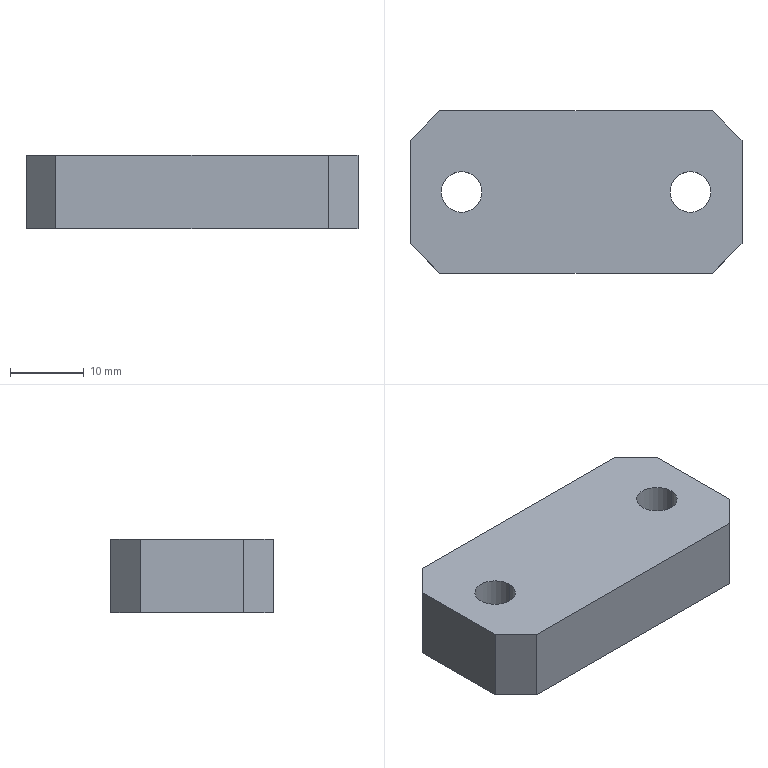Part | Creo | 1 solid | 20 faces | box 45 x 22 x 10 mm | volume 8539 mm3 | plane 12 | cylinder 8 | commonest cylinder face diameters 5.5 x4 9.5 x4
STEP:
#1=CARTESIAN_POINT('',(-202.734,-76.26,-294.5));
#2=VERTEX_POINT('',#1);
#3=CARTESIAN_POINT('',(-165.734,-76.26,-294.5));
#4=VERTEX_POINT('',#3);
#5=CARTESIAN_POINT('',(-202.734,-76.26,-294.5));
#6=DIRECTION('',(1.,0.,0.));
#7=VECTOR('',#6,37.);
#8=LINE('',#5,#7);
#9=EDGE_CURVE('',#2,#4,#8,.T.);
#10=ORIENTED_EDGE('',*,*,#9,.F.);
#11=CARTESIAN_POINT('',(-206.734,-72.26,-294.5));
#12=VERTEX_POINT('',#11);
#13=CARTESIAN_POINT('',(-206.734,-72.26,-294.5));
#14=DIRECTION('',(0.7071,-0.7071,0.));
#15=VECTOR('',#14,5.657);
#16=LINE('',#13,#15);
#17=EDGE_CURVE('',#12,#2,#16,.T.);
#18=ORIENTED_EDGE('',*,*,#17,.F.);
#19=CARTESIAN_POINT('',(-206.734,-58.26,-294.5));
#20=VERTEX_POINT('',#19);
#21=CARTESIAN_POINT('',(-206.734,-72.26,-294.5));
#22=DIRECTION('',(0.,1.,0.));
#23=VECTOR('',#22,14.);
#24=LINE('',#21,#23);
#25=EDGE_CURVE('',#12,#20,#24,.T.);
#26=ORIENTED_EDGE('',*,*,#25,.T.);
#27=CARTESIAN_POINT('',(-202.734,-54.26,-294.5));
#28=VERTEX_POINT('',#27);
#29=CARTESIAN_POINT('',(-202.734,-54.26,-294.5));
#30=DIRECTION('',(-0.7071,-0.7071,0.));
#31=VECTOR('',#30,5.657);
#32=LINE('',#29,#31);
#33=EDGE_CURVE('',#28,#20,#32,.T.);
#34=ORIENTED_EDGE('',*,*,#33,.F.);
#35=CARTESIAN_POINT('',(-165.734,-54.26,-294.5));
#36=VERTEX_POINT('',#35);
#37=CARTESIAN_POINT('',(-165.734,-54.26,-294.5));
#38=DIRECTION('',(-1.,0.,0.));
#39=VECTOR('',#38,37.);
#40=LINE('',#37,#39);
#41=EDGE_CURVE('',#36,#28,#40,.T.);
#42=ORIENTED_EDGE('',*,*,#41,.F.);
#43=CARTESIAN_POINT('',(-161.734,-58.26,-294.5));
#44=VERTEX_POINT('',#43);
#45=CARTESIAN_POINT('',(-161.734,-58.26,-294.5));
#46=DIRECTION('',(-0.7071,0.7071,0.));
#47=VECTOR('',#46,5.657);
#48=LINE('',#45,#47);
#49=EDGE_CURVE('',#44,#36,#48,.T.);
#50=ORIENTED_EDGE('',*,*,#49,.F.);
#51=CARTESIAN_POINT('',(-161.734,-72.26,-294.5));
#52=VERTEX_POINT('',#51);
#53=CARTESIAN_POINT('',(-161.734,-72.26,-294.5));
#54=DIRECTION('',(0.,1.,0.));
#55=VECTOR('',#54,14.);
#56=LINE('',#53,#55);
#57=EDGE_CURVE('',#52,#44,#56,.T.);
#58=ORIENTED_EDGE('',*,*,#57,.F.);
#59=CARTESIAN_POINT('',(-165.734,-76.26,-294.5));
#60=DIRECTION('',(0.7071,0.7071,0.));
#61=VECTOR('',#60,5.657);
#62=LINE('',#59,#61);
#63=EDGE_CURVE('',#4,#52,#62,.T.);
#64=ORIENTED_EDGE('',*,*,#63,.F.);
#65=EDGE_LOOP('',(#10,#18,#26,#34,#42,#50,#58,#64));
#66=FACE_OUTER_BOUND('',#65,.F.);
#67=CARTESIAN_POINT('',(-196.984,-65.26,-294.5));
#68=VERTEX_POINT('',#67);
#69=CARTESIAN_POINT('',(-202.484,-65.26,-294.5));
#70=VERTEX_POINT('',#69);
#71=CARTESIAN_POINT('',(-199.734,-65.26,-294.5));
#72=DIRECTION('',(0.,0.,-1.));
#73=DIRECTION('',(1.,0.,0.));
#74=AXIS2_PLACEMENT_3D('',#71,#72,#73);
#75=CIRCLE('',#74,2.75);
#76=EDGE_CURVE('',#68,#70,#75,.T.);
#77=ORIENTED_EDGE('',*,*,#76,.F.);
#78=CARTESIAN_POINT('',(-199.734,-65.26,-294.5));
#79=DIRECTION('',(0.,0.,-1.));
#80=DIRECTION('',(-1.,0.,0.));
#81=AXIS2_PLACEMENT_3D('',#78,#79,#80);
#82=CIRCLE('',#81,2.75);
#83=EDGE_CURVE('',#70,#68,#82,.T.);
#84=ORIENTED_EDGE('',*,*,#83,.F.);
#85=EDGE_LOOP('',(#77,#84));
#86=FACE_BOUND('',#85,.F.);
#87=CARTESIAN_POINT('',(-165.984,-65.26,-294.5));
#88=VERTEX_POINT('',#87);
#89=CARTESIAN_POINT('',(-171.484,-65.26,-294.5));
#90=VERTEX_POINT('',#89);
#91=CARTESIAN_POINT('',(-168.734,-65.26,-294.5));
#92=DIRECTION('',(0.,0.,-1.));
#93=DIRECTION('',(1.,0.,0.));
#94=AXIS2_PLACEMENT_3D('',#91,#92,#93);
#95=CIRCLE('',#94,2.75);
#96=EDGE_CURVE('',#88,#90,#95,.T.);
#97=ORIENTED_EDGE('',*,*,#96,.F.);
#98=CARTESIAN_POINT('',(-168.734,-65.26,-294.5));
#99=DIRECTION('',(0.,0.,-1.));
#100=DIRECTION('',(-1.,0.,0.));
#101=AXIS2_PLACEMENT_3D('',#98,#99,#100);
#102=CIRCLE('',#101,2.75);
#103=EDGE_CURVE('',#90,#88,#102,.T.);
#104=ORIENTED_EDGE('',*,*,#103,.F.);
#105=EDGE_LOOP('',(#97,#104));
#106=FACE_BOUND('',#105,.F.);
#107=CARTESIAN_POINT('',(-177.734,-55.26,-294.5));
#108=DIRECTION('',(0.,0.,1.));
#109=DIRECTION('',(-1.,0.,0.));
#110=AXIS2_PLACEMENT_3D('',#107,#108,#109);
#111=PLANE('',#110);
#112=ADVANCED_FACE('',(#66,#86,#106),#111,.T.);
#113=CARTESIAN_POINT('',(-202.484,-65.26,-298.5));
#114=VERTEX_POINT('',#113);
#115=CARTESIAN_POINT('',(-196.984,-65.26,-298.5));
#116=VERTEX_POINT('',#115);
#117=CARTESIAN_POINT('',(-199.734,-65.26,-298.5));
#118=DIRECTION('',(0.,0.,1.));
#119=DIRECTION('',(-1.,0.,0.));
#120=AXIS2_PLACEMENT_3D('',#117,#118,#119);
#121=CIRCLE('',#120,2.75);
#122=EDGE_CURVE('',#114,#116,#121,.T.);
#123=ORIENTED_EDGE('',*,*,#122,.T.);
#124=CARTESIAN_POINT('',(-196.984,-65.26,-294.5));
#125=DIRECTION('',(0.,0.,-1.));
#126=VECTOR('',#125,4.);
#127=LINE('',#124,#126);
#128=EDGE_CURVE('',#68,#116,#127,.T.);
#129=ORIENTED_EDGE('',*,*,#128,.F.);
#130=ORIENTED_EDGE('',*,*,#76,.T.);
#131=CARTESIAN_POINT('',(-202.484,-65.26,-294.5));
#132=DIRECTION('',(0.,0.,-1.));
#133=VECTOR('',#132,4.);
#134=LINE('',#131,#133);
#135=EDGE_CURVE('',#70,#114,#134,.T.);
#136=ORIENTED_EDGE('',*,*,#135,.T.);
#137=EDGE_LOOP('',(#123,#129,#130,#136));
#138=FACE_OUTER_BOUND('',#137,.F.);
#139=CARTESIAN_POINT('',(-199.734,-65.26,-294.5));
#140=DIRECTION('',(0.,0.,-1.));
#141=DIRECTION('',(1.,0.,0.));
#142=AXIS2_PLACEMENT_3D('',#139,#140,#141);
#143=CYLINDRICAL_SURFACE('',#142,2.75);
#144=ADVANCED_FACE('',(#138),#143,.F.);
#145=CARTESIAN_POINT('',(-194.984,-65.26,-298.5));
#146=VERTEX_POINT('',#145);
#147=CARTESIAN_POINT('',(-204.484,-65.26,-298.5));
#148=VERTEX_POINT('',#147);
#149=CARTESIAN_POINT('',(-199.734,-65.26,-298.5));
#150=DIRECTION('',(0.,0.,-1.));
#151=DIRECTION('',(1.,0.,0.));
#152=AXIS2_PLACEMENT_3D('',#149,#150,#151);
#153=CIRCLE('',#152,4.75);
#154=EDGE_CURVE('',#146,#148,#153,.T.);
#155=ORIENTED_EDGE('',*,*,#154,.F.);
#156=CARTESIAN_POINT('',(-199.734,-65.26,-298.5));
#157=DIRECTION('',(0.,0.,-1.));
#158=DIRECTION('',(-1.,0.,0.));
#159=AXIS2_PLACEMENT_3D('',#156,#157,#158);
#160=CIRCLE('',#159,4.75);
#161=EDGE_CURVE('',#148,#146,#160,.T.);
#162=ORIENTED_EDGE('',*,*,#161,.F.);
#163=EDGE_LOOP('',(#155,#162));
#164=FACE_OUTER_BOUND('',#163,.F.);
#165=CARTESIAN_POINT('',(-199.734,-65.26,-298.5));
#166=DIRECTION('',(0.,0.,1.));
#167=DIRECTION('',(1.,0.,0.));
#168=AXIS2_PLACEMENT_3D('',#165,#166,#167);
#169=CIRCLE('',#168,2.75);
#170=EDGE_CURVE('',#116,#114,#169,.T.);
#171=ORIENTED_EDGE('',*,*,#170,.F.);
#172=ORIENTED_EDGE('',*,*,#122,.F.);
#173=EDGE_LOOP('',(#171,#172));
#174=FACE_BOUND('',#173,.F.);
#175=CARTESIAN_POINT('',(-199.734,-65.26,-298.5));
#176=DIRECTION('',(0.,0.,1.));
#177=DIRECTION('',(-1.,0.,0.));
#178=AXIS2_PLACEMENT_3D('',#175,#176,#177);
#179=PLANE('',#178);
#180=ADVANCED_FACE('',(#164,#174),#179,.F.);
#181=ORIENTED_EDGE('',*,*,#170,.T.);
#182=ORIENTED_EDGE('',*,*,#135,.F.);
#183=ORIENTED_EDGE('',*,*,#83,.T.);
#184=ORIENTED_EDGE('',*,*,#128,.T.);
#185=EDGE_LOOP('',(#181,#182,#183,#184));
#186=FACE_OUTER_BOUND('',#185,.F.);
#187=CARTESIAN_POINT('',(-199.734,-65.26,-294.5));
#188=DIRECTION('',(0.,0.,-1.));
#189=DIRECTION('',(1.,0.,0.));
#190=AXIS2_PLACEMENT_3D('',#187,#188,#189);
#191=CYLINDRICAL_SURFACE('',#190,2.75);
#192=ADVANCED_FACE('',(#186),#191,.F.);
#193=CARTESIAN_POINT('',(-204.484,-65.26,-304.5));
#194=VERTEX_POINT('',#193);
#195=CARTESIAN_POINT('',(-194.984,-65.26,-304.5));
#196=VERTEX_POINT('',#195);
#197=CARTESIAN_POINT('',(-199.734,-65.26,-304.5));
#198=DIRECTION('',(0.,0.,1.));
#199=DIRECTION('',(-1.,0.,0.));
#200=AXIS2_PLACEMENT_3D('',#197,#198,#199);
#201=CIRCLE('',#200,4.75);
#202=EDGE_CURVE('',#194,#196,#201,.T.);
#203=ORIENTED_EDGE('',*,*,#202,.T.);
#204=CARTESIAN_POINT('',(-194.984,-65.26,-298.5));
#205=DIRECTION('',(0.,0.,-1.));
#206=VECTOR('',#205,6.);
#207=LINE('',#204,#206);
#208=EDGE_CURVE('',#146,#196,#207,.T.);
#209=ORIENTED_EDGE('',*,*,#208,.F.);
#210=ORIENTED_EDGE('',*,*,#154,.T.);
#211=CARTESIAN_POINT('',(-204.484,-65.26,-298.5));
#212=DIRECTION('',(0.,0.,-1.));
#213=VECTOR('',#212,6.);
#214=LINE('',#211,#213);
#215=EDGE_CURVE('',#148,#194,#214,.T.);
#216=ORIENTED_EDGE('',*,*,#215,.T.);
#217=EDGE_LOOP('',(#203,#209,#210,#216));
#218=FACE_OUTER_BOUND('',#217,.F.);
#219=CARTESIAN_POINT('',(-199.734,-65.26,-298.5));
#220=DIRECTION('',(0.,0.,-1.));
#221=DIRECTION('',(1.,0.,0.));
#222=AXIS2_PLACEMENT_3D('',#219,#220,#221);
#223=CYLINDRICAL_SURFACE('',#222,4.75);
#224=ADVANCED_FACE('',(#218),#223,.F.);
#225=CARTESIAN_POINT('',(-206.734,-58.26,-304.5));
#226=VERTEX_POINT('',#225);
#227=CARTESIAN_POINT('',(-206.734,-72.26,-304.5));
#228=VERTEX_POINT('',#227);
#229=CARTESIAN_POINT('',(-206.734,-58.26,-304.5));
#230=DIRECTION('',(0.,-1.,0.));
#231=VECTOR('',#230,14.);
#232=LINE('',#229,#231);
#233=EDGE_CURVE('',#226,#228,#232,.T.);
#234=ORIENTED_EDGE('',*,*,#233,.T.);
#235=CARTESIAN_POINT('',(-202.734,-76.26,-304.5));
#236=VERTEX_POINT('',#235);
#237=CARTESIAN_POINT('',(-202.734,-76.26,-304.5));
#238=DIRECTION('',(-0.7071,0.7071,0.));
#239=VECTOR('',#238,5.657);
#240=LINE('',#237,#239);
#241=EDGE_CURVE('',#236,#228,#240,.T.);
#242=ORIENTED_EDGE('',*,*,#241,.F.);
#243=CARTESIAN_POINT('',(-165.734,-76.26,-304.5));
#244=VERTEX_POINT('',#243);
#245=CARTESIAN_POINT('',(-165.734,-76.26,-304.5));
#246=DIRECTION('',(-1.,0.,0.));
#247=VECTOR('',#246,37.);
#248=LINE('',#245,#247);
#249=EDGE_CURVE('',#244,#236,#248,.T.);
#250=ORIENTED_EDGE('',*,*,#249,.F.);
#251=CARTESIAN_POINT('',(-161.734,-72.26,-304.5));
#252=VERTEX_POINT('',#251);
#253=CARTESIAN_POINT('',(-161.734,-72.26,-304.5));
#254=DIRECTION('',(-0.7071,-0.7071,0.));
#255=VECTOR('',#254,5.657);
#256=LINE('',#253,#255);
#257=EDGE_CURVE('',#252,#244,#256,.T.);
#258=ORIENTED_EDGE('',*,*,#257,.F.);
#259=CARTESIAN_POINT('',(-161.734,-58.26,-304.5));
#260=VERTEX_POINT('',#259);
#261=CARTESIAN_POINT('',(-161.734,-58.26,-304.5));
#262=DIRECTION('',(0.,-1.,0.));
#263=VECTOR('',#262,14.);
#264=LINE('',#261,#263);
#265=EDGE_CURVE('',#260,#252,#264,.T.);
#266=ORIENTED_EDGE('',*,*,#265,.F.);
#267=CARTESIAN_POINT('',(-165.734,-54.26,-304.5));
#268=VERTEX_POINT('',#267);
#269=CARTESIAN_POINT('',(-165.734,-54.26,-304.5));
#270=DIRECTION('',(0.7071,-0.7071,0.));
#271=VECTOR('',#270,5.657);
#272=LINE('',#269,#271);
#273=EDGE_CURVE('',#268,#260,#272,.T.);
#274=ORIENTED_EDGE('',*,*,#273,.F.);
#275=CARTESIAN_POINT('',(-202.734,-54.26,-304.5));
#276=VERTEX_POINT('',#275);
#277=CARTESIAN_POINT('',(-202.734,-54.26,-304.5));
#278=DIRECTION('',(1.,0.,0.));
#279=VECTOR('',#278,37.);
#280=LINE('',#277,#279);
#281=EDGE_CURVE('',#276,#268,#280,.T.);
#282=ORIENTED_EDGE('',*,*,#281,.F.);
#283=CARTESIAN_POINT('',(-206.734,-58.26,-304.5));
#284=DIRECTION('',(0.7071,0.7071,0.));
#285=VECTOR('',#284,5.657);
#286=LINE('',#283,#285);
#287=EDGE_CURVE('',#226,#276,#286,.T.);
#288=ORIENTED_EDGE('',*,*,#287,.F.);
#289=EDGE_LOOP('',(#234,#242,#250,#258,#266,#274,#282,#288));
#290=FACE_OUTER_BOUND('',#289,.F.);
#291=CARTESIAN_POINT('',(-199.734,-65.26,-304.5));
#292=DIRECTION('',(0.,0.,1.));
#293=DIRECTION('',(1.,0.,0.));
#294=AXIS2_PLACEMENT_3D('',#291,#292,#293);
#295=CIRCLE('',#294,4.75);
#296=EDGE_CURVE('',#196,#194,#295,.T.);
#297=ORIENTED_EDGE('',*,*,#296,.F.);
#298=ORIENTED_EDGE('',*,*,#202,.F.);
#299=EDGE_LOOP('',(#297,#298));
#300=FACE_BOUND('',#299,.F.);
#301=CARTESIAN_POINT('',(-163.984,-65.26,-304.5));
#302=VERTEX_POINT('',#301);
#303=CARTESIAN_POINT('',(-173.484,-65.26,-304.5));
#304=VERTEX_POINT('',#303);
#305=CARTESIAN_POINT('',(-168.734,-65.26,-304.5));
#306=DIRECTION('',(0.,0.,1.));
#307=DIRECTION('',(1.,0.,0.));
#308=AXIS2_PLACEMENT_3D('',#305,#306,#307);
#309=CIRCLE('',#308,4.75);
#310=EDGE_CURVE('',#302,#304,#309,.T.);
#311=ORIENTED_EDGE('',*,*,#310,.F.);
#312=CARTESIAN_POINT('',(-168.734,-65.26,-304.5));
#313=DIRECTION('',(0.,0.,1.));
#314=DIRECTION('',(-1.,0.,0.));
#315=AXIS2_PLACEMENT_3D('',#312,#313,#314);
#316=CIRCLE('',#315,4.75);
#317=EDGE_CURVE('',#304,#302,#316,.T.);
#318=ORIENTED_EDGE('',*,*,#317,.F.);
#319=EDGE_LOOP('',(#311,#318));
#320=FACE_BOUND('',#319,.F.);
#321=CARTESIAN_POINT('',(-177.734,-55.26,-304.5));
#322=DIRECTION('',(0.,0.,-1.));
#323=DIRECTION('',(1.,0.,0.));
#324=AXIS2_PLACEMENT_3D('',#321,#322,#323);
#325=PLANE('',#324);
#326=ADVANCED_FACE('',(#290,#300,#320),#325,.T.);
#327=ORIENTED_EDGE('',*,*,#310,.T.);
#328=CARTESIAN_POINT('',(-173.484,-65.26,-298.5));
#329=VERTEX_POINT('',#328);
#330=CARTESIAN_POINT('',(-173.484,-65.26,-298.5));
#331=DIRECTION('',(0.,0.,-1.));
#332=VECTOR('',#331,6.);
#333=LINE('',#330,#332);
#334=EDGE_CURVE('',#329,#304,#333,.T.);
#335=ORIENTED_EDGE('',*,*,#334,.F.);
#336=CARTESIAN_POINT('',(-163.984,-65.26,-298.5));
#337=VERTEX_POINT('',#336);
#338=CARTESIAN_POINT('',(-168.734,-65.26,-298.5));
#339=DIRECTION('',(0.,0.,-1.));
#340=DIRECTION('',(-1.,0.,0.));
#341=AXIS2_PLACEMENT_3D('',#338,#339,#340);
#342=CIRCLE('',#341,4.75);
#343=EDGE_CURVE('',#329,#337,#342,.T.);
#344=ORIENTED_EDGE('',*,*,#343,.T.);
#345=CARTESIAN_POINT('',(-163.984,-65.26,-298.5));
#346=DIRECTION('',(0.,0.,-1.));
#347=VECTOR('',#346,6.);
#348=LINE('',#345,#347);
#349=EDGE_CURVE('',#337,#302,#348,.T.);
#350=ORIENTED_EDGE('',*,*,#349,.T.);
#351=EDGE_LOOP('',(#327,#335,#344,#350));
#352=FACE_OUTER_BOUND('',#351,.F.);
#353=CARTESIAN_POINT('',(-168.734,-65.26,-298.5));
#354=DIRECTION('',(0.,0.,-1.));
#355=DIRECTION('',(1.,0.,0.));
#356=AXIS2_PLACEMENT_3D('',#353,#354,#355);
#357=CYLINDRICAL_SURFACE('',#356,4.75);
#358=ADVANCED_FACE('',(#352),#357,.F.);
#359=ORIENTED_EDGE('',*,*,#317,.T.);
#360=ORIENTED_EDGE('',*,*,#349,.F.);
#361=CARTESIAN_POINT('',(-168.734,-65.26,-298.5));
#362=DIRECTION('',(0.,0.,-1.));
#363=DIRECTION('',(1.,0.,0.));
#364=AXIS2_PLACEMENT_3D('',#361,#362,#363);
#365=CIRCLE('',#364,4.75);
#366=EDGE_CURVE('',#337,#329,#365,.T.);
#367=ORIENTED_EDGE('',*,*,#366,.T.);
#368=ORIENTED_EDGE('',*,*,#334,.T.);
#369=EDGE_LOOP('',(#359,#360,#367,#368));
#370=FACE_OUTER_BOUND('',#369,.F.);
#371=CARTESIAN_POINT('',(-168.734,-65.26,-298.5));
#372=DIRECTION('',(0.,0.,-1.));
#373=DIRECTION('',(1.,0.,0.));
#374=AXIS2_PLACEMENT_3D('',#371,#372,#373);
#375=CYLINDRICAL_SURFACE('',#374,4.75);
#376=ADVANCED_FACE('',(#370),#375,.F.);
#377=ORIENTED_EDGE('',*,*,#366,.F.);
#378=ORIENTED_EDGE('',*,*,#343,.F.);
#379=EDGE_LOOP('',(#377,#378));
#380=FACE_OUTER_BOUND('',#379,.F.);
#381=CARTESIAN_POINT('',(-165.984,-65.26,-298.5));
#382=VERTEX_POINT('',#381);
#383=CARTESIAN_POINT('',(-171.484,-65.26,-298.5));
#384=VERTEX_POINT('',#383);
#385=CARTESIAN_POINT('',(-168.734,-65.26,-298.5));
#386=DIRECTION('',(0.,0.,1.));
#387=DIRECTION('',(1.,0.,0.));
#388=AXIS2_PLACEMENT_3D('',#385,#386,#387);
#389=CIRCLE('',#388,2.75);
#390=EDGE_CURVE('',#382,#384,#389,.T.);
#391=ORIENTED_EDGE('',*,*,#390,.F.);
#392=CARTESIAN_POINT('',(-168.734,-65.26,-298.5));
#393=DIRECTION('',(0.,0.,1.));
#394=DIRECTION('',(-1.,0.,0.));
#395=AXIS2_PLACEMENT_3D('',#392,#393,#394);
#396=CIRCLE('',#395,2.75);
#397=EDGE_CURVE('',#384,#382,#396,.T.);
#398=ORIENTED_EDGE('',*,*,#397,.F.);
#399=EDGE_LOOP('',(#391,#398));
#400=FACE_BOUND('',#399,.F.);
#401=CARTESIAN_POINT('',(-168.734,-65.26,-298.5));
#402=DIRECTION('',(0.,0.,1.));
#403=DIRECTION('',(-1.,0.,0.));
#404=AXIS2_PLACEMENT_3D('',#401,#402,#403);
#405=PLANE('',#404);
#406=ADVANCED_FACE('',(#380,#400),#405,.F.);
#407=ORIENTED_EDGE('',*,*,#390,.T.);
#408=CARTESIAN_POINT('',(-171.484,-65.26,-294.5));
#409=DIRECTION('',(0.,0.,-1.));
#410=VECTOR('',#409,4.);
#411=LINE('',#408,#410);
#412=EDGE_CURVE('',#90,#384,#411,.T.);
#413=ORIENTED_EDGE('',*,*,#412,.F.);
#414=ORIENTED_EDGE('',*,*,#103,.T.);
#415=CARTESIAN_POINT('',(-165.984,-65.26,-294.5));
#416=DIRECTION('',(0.,0.,-1.));
#417=VECTOR('',#416,4.);
#418=LINE('',#415,#417);
#419=EDGE_CURVE('',#88,#382,#418,.T.);
#420=ORIENTED_EDGE('',*,*,#419,.T.);
#421=EDGE_LOOP('',(#407,#413,#414,#420));
#422=FACE_OUTER_BOUND('',#421,.F.);
#423=CARTESIAN_POINT('',(-168.734,-65.26,-294.5));
#424=DIRECTION('',(0.,0.,-1.));
#425=DIRECTION('',(1.,0.,0.));
#426=AXIS2_PLACEMENT_3D('',#423,#424,#425);
#427=CYLINDRICAL_SURFACE('',#426,2.75);
#428=ADVANCED_FACE('',(#422),#427,.F.);
#429=ORIENTED_EDGE('',*,*,#397,.T.);
#430=ORIENTED_EDGE('',*,*,#419,.F.);
#431=ORIENTED_EDGE('',*,*,#96,.T.);
#432=ORIENTED_EDGE('',*,*,#412,.T.);
#433=EDGE_LOOP('',(#429,#430,#431,#432));
#434=FACE_OUTER_BOUND('',#433,.F.);
#435=CARTESIAN_POINT('',(-168.734,-65.26,-294.5));
#436=DIRECTION('',(0.,0.,-1.));
#437=DIRECTION('',(1.,0.,0.));
#438=AXIS2_PLACEMENT_3D('',#435,#436,#437);
#439=CYLINDRICAL_SURFACE('',#438,2.75);
#440=ADVANCED_FACE('',(#434),#439,.F.);
#441=ORIENTED_EDGE('',*,*,#296,.T.);
#442=ORIENTED_EDGE('',*,*,#215,.F.);
#443=ORIENTED_EDGE('',*,*,#161,.T.);
#444=ORIENTED_EDGE('',*,*,#208,.T.);
#445=EDGE_LOOP('',(#441,#442,#443,#444));
#446=FACE_OUTER_BOUND('',#445,.F.);
#447=CARTESIAN_POINT('',(-199.734,-65.26,-298.5));
#448=DIRECTION('',(0.,0.,-1.));
#449=DIRECTION('',(1.,0.,0.));
#450=AXIS2_PLACEMENT_3D('',#447,#448,#449);
#451=CYLINDRICAL_SURFACE('',#450,4.75);
#452=ADVANCED_FACE('',(#446),#451,.F.);
#453=ORIENTED_EDGE('',*,*,#25,.F.);
#454=CARTESIAN_POINT('',(-206.734,-72.26,-304.5));
#455=DIRECTION('',(0.,0.,1.));
#456=VECTOR('',#455,10.);
#457=LINE('',#454,#456);
#458=EDGE_CURVE('',#228,#12,#457,.T.);
#459=ORIENTED_EDGE('',*,*,#458,.F.);
#460=ORIENTED_EDGE('',*,*,#233,.F.);
#461=CARTESIAN_POINT('',(-206.734,-58.26,-294.5));
#462=DIRECTION('',(0.,0.,-1.));
#463=VECTOR('',#462,10.);
#464=LINE('',#461,#463);
#465=EDGE_CURVE('',#20,#226,#464,.T.);
#466=ORIENTED_EDGE('',*,*,#465,.F.);
#467=EDGE_LOOP('',(#453,#459,#460,#466));
#468=FACE_OUTER_BOUND('',#467,.F.);
#469=CARTESIAN_POINT('',(-206.734,-53.26,-299.5));
#470=DIRECTION('',(1.,0.,0.));
#471=DIRECTION('',(0.,0.,-1.));
#472=AXIS2_PLACEMENT_3D('',#469,#470,#471);
#473=PLANE('',#472);
#474=ADVANCED_FACE('',(#468),#473,.F.);
#475=ORIENTED_EDGE('',*,*,#241,.T.);
#476=ORIENTED_EDGE('',*,*,#458,.T.);
#477=ORIENTED_EDGE('',*,*,#17,.T.);
#478=CARTESIAN_POINT('',(-202.734,-76.26,-294.5));
#479=DIRECTION('',(0.,0.,-1.));
#480=VECTOR('',#479,10.);
#481=LINE('',#478,#480);
#482=EDGE_CURVE('',#2,#236,#481,.T.);
#483=ORIENTED_EDGE('',*,*,#482,.T.);
#484=EDGE_LOOP('',(#475,#476,#477,#483));
#485=FACE_OUTER_BOUND('',#484,.F.);
#486=CARTESIAN_POINT('',(-202.734,-76.26,-299.5));
#487=DIRECTION('',(0.7071,0.7071,0.));
#488=DIRECTION('',(0.7071,-0.7071,0.));
#489=AXIS2_PLACEMENT_3D('',#486,#487,#488);
#490=PLANE('',#489);
#491=ADVANCED_FACE('',(#485),#490,.F.);
#492=ORIENTED_EDGE('',*,*,#249,.T.);
#493=ORIENTED_EDGE('',*,*,#482,.F.);
#494=ORIENTED_EDGE('',*,*,#9,.T.);
#495=CARTESIAN_POINT('',(-165.734,-76.26,-304.5));
#496=DIRECTION('',(0.,0.,1.));
#497=VECTOR('',#496,10.);
#498=LINE('',#495,#497);
#499=EDGE_CURVE('',#244,#4,#498,.T.);
#500=ORIENTED_EDGE('',*,*,#499,.F.);
#501=EDGE_LOOP('',(#492,#493,#494,#500));
#502=FACE_OUTER_BOUND('',#501,.F.);
#503=CARTESIAN_POINT('',(-195.484,-76.26,-299.5));
#504=DIRECTION('',(0.,1.,0.));
#505=DIRECTION('',(0.,0.,1.));
#506=AXIS2_PLACEMENT_3D('',#503,#504,#505);
#507=PLANE('',#506);
#508=ADVANCED_FACE('',(#502),#507,.F.);
#509=ORIENTED_EDGE('',*,*,#257,.T.);
#510=ORIENTED_EDGE('',*,*,#499,.T.);
#511=ORIENTED_EDGE('',*,*,#63,.T.);
#512=CARTESIAN_POINT('',(-161.734,-72.26,-294.5));
#513=DIRECTION('',(0.,0.,-1.));
#514=VECTOR('',#513,10.);
#515=LINE('',#512,#514);
#516=EDGE_CURVE('',#52,#252,#515,.T.);
#517=ORIENTED_EDGE('',*,*,#516,.T.);
#518=EDGE_LOOP('',(#509,#510,#511,#517));
#519=FACE_OUTER_BOUND('',#518,.F.);
#520=CARTESIAN_POINT('',(-161.734,-72.26,-299.5));
#521=DIRECTION('',(-0.7071,0.7071,0.));
#522=DIRECTION('',(0.7071,0.7071,0.));
#523=AXIS2_PLACEMENT_3D('',#520,#521,#522);
#524=PLANE('',#523);
#525=ADVANCED_FACE('',(#519),#524,.F.);
#526=ORIENTED_EDGE('',*,*,#57,.T.);
#527=CARTESIAN_POINT('',(-161.734,-58.26,-304.5));
#528=DIRECTION('',(0.,0.,1.));
#529=VECTOR('',#528,10.);
#530=LINE('',#527,#529);
#531=EDGE_CURVE('',#260,#44,#530,.T.);
#532=ORIENTED_EDGE('',*,*,#531,.F.);
#533=ORIENTED_EDGE('',*,*,#265,.T.);
#534=ORIENTED_EDGE('',*,*,#516,.F.);
#535=EDGE_LOOP('',(#526,#532,#533,#534));
#536=FACE_OUTER_BOUND('',#535,.F.);
#537=CARTESIAN_POINT('',(-161.734,-53.26,-299.5));
#538=DIRECTION('',(-1.,0.,0.));
#539=DIRECTION('',(0.,0.,-1.));
#540=AXIS2_PLACEMENT_3D('',#537,#538,#539);
#541=PLANE('',#540);
#542=ADVANCED_FACE('',(#536),#541,.F.);
#543=ORIENTED_EDGE('',*,*,#273,.T.);
#544=ORIENTED_EDGE('',*,*,#531,.T.);
#545=ORIENTED_EDGE('',*,*,#49,.T.);
#546=CARTESIAN_POINT('',(-165.734,-54.26,-294.5));
#547=DIRECTION('',(0.,0.,-1.));
#548=VECTOR('',#547,10.);
#549=LINE('',#546,#548);
#550=EDGE_CURVE('',#36,#268,#549,.T.);
#551=ORIENTED_EDGE('',*,*,#550,.T.);
#552=EDGE_LOOP('',(#543,#544,#545,#551));
#553=FACE_OUTER_BOUND('',#552,.F.);
#554=CARTESIAN_POINT('',(-165.734,-54.26,-299.5));
#555=DIRECTION('',(-0.7071,-0.7071,0.));
#556=DIRECTION('',(-0.7071,0.7071,0.));
#557=AXIS2_PLACEMENT_3D('',#554,#555,#556);
#558=PLANE('',#557);
#559=ADVANCED_FACE('',(#553),#558,.F.);
#560=ORIENTED_EDGE('',*,*,#41,.T.);
#561=CARTESIAN_POINT('',(-202.734,-54.26,-304.5));
#562=DIRECTION('',(0.,0.,1.));
#563=VECTOR('',#562,10.);
#564=LINE('',#561,#563);
#565=EDGE_CURVE('',#276,#28,#564,.T.);
#566=ORIENTED_EDGE('',*,*,#565,.F.);
#567=ORIENTED_EDGE('',*,*,#281,.T.);
#568=ORIENTED_EDGE('',*,*,#550,.F.);
#569=EDGE_LOOP('',(#560,#566,#567,#568));
#570=FACE_OUTER_BOUND('',#569,.F.);
#571=CARTESIAN_POINT('',(-172.984,-54.26,-299.5));
#572=DIRECTION('',(0.,-1.,0.));
#573=DIRECTION('',(0.,0.,1.));
#574=AXIS2_PLACEMENT_3D('',#571,#572,#573);
#575=PLANE('',#574);
#576=ADVANCED_FACE('',(#570),#575,.F.);
#577=ORIENTED_EDGE('',*,*,#287,.T.);
#578=ORIENTED_EDGE('',*,*,#565,.T.);
#579=ORIENTED_EDGE('',*,*,#33,.T.);
#580=ORIENTED_EDGE('',*,*,#465,.T.);
#581=EDGE_LOOP('',(#577,#578,#579,#580));
#582=FACE_OUTER_BOUND('',#581,.F.);
#583=CARTESIAN_POINT('',(-206.734,-58.26,-299.5));
#584=DIRECTION('',(0.7071,-0.7071,0.));
#585=DIRECTION('',(-0.7071,-0.7071,0.));
#586=AXIS2_PLACEMENT_3D('',#583,#584,#585);
#587=PLANE('',#586);
#588=ADVANCED_FACE('',(#582),#587,.F.);
#589=CLOSED_SHELL('',(#112,#144,#180,#192,#224,#326,#358,#376,#406,#428,#440,#452,#474,#491,#508,#525,#542,#559,#576,#588));
#590=MANIFOLD_SOLID_BREP('',#589);
#591=(LENGTH_UNIT()NAMED_UNIT(*)SI_UNIT(.MILLI.,.METRE.));
#592=UNCERTAINTY_MEASURE_WITH_UNIT(LENGTH_MEASURE(0.005108),#591,'','');
#593=(NAMED_UNIT(*)PLANE_ANGLE_UNIT()SI_UNIT($,.RADIAN.));
#594=PLANE_ANGLE_MEASURE_WITH_UNIT(PLANE_ANGLE_MEASURE(0.01745),#593);
#595=(CONVERSION_BASED_UNIT('DEGREE',#594)NAMED_UNIT(*)PLANE_ANGLE_UNIT());
#596=(NAMED_UNIT(*)SI_UNIT($,.STERADIAN.)SOLID_ANGLE_UNIT());
#597=(GEOMETRIC_REPRESENTATION_CONTEXT(3)GLOBAL_UNCERTAINTY_ASSIGNED_CONTEXT((#592))GLOBAL_UNIT_ASSIGNED_CONTEXT((#591,#595,#596))REPRESENTATION_CONTEXT('',''));
#598=ADVANCED_BREP_SHAPE_REPRESENTATION('',(#590),#597);